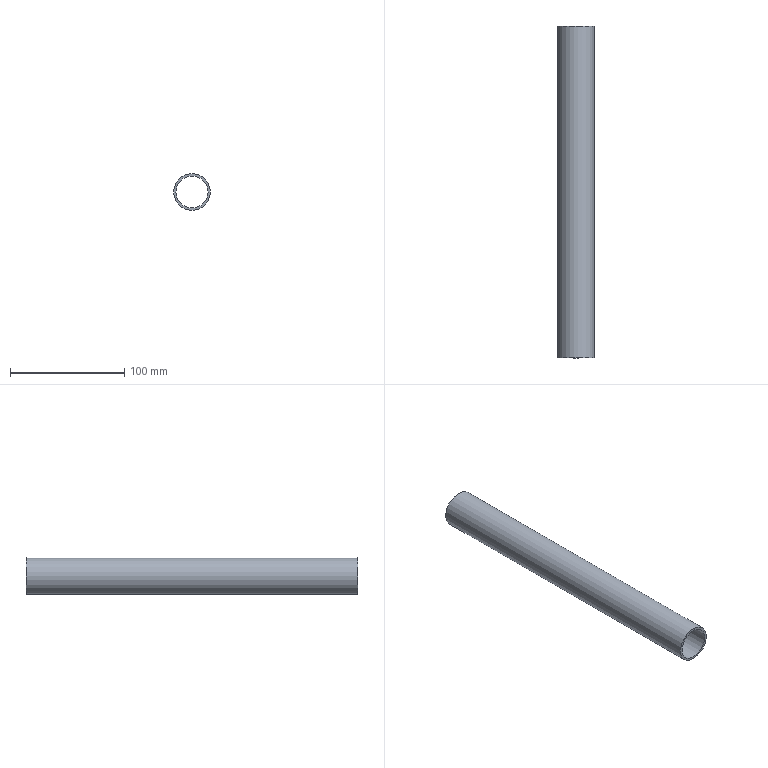Part | STEP file | 1-56.16 | 1 solid | 4 faces | box 32 x 290 x 32 mm | volume 54664 mm3 | plane 2 | cylinder 2 | commonest cylinder face diameters 28 x1 32 x1
STEP:
#1=CARTESIAN_POINT('',(0.,0.,0.));
#2=DIRECTION('',(0.,0.,1.));
#3=DIRECTION('',(1.,0.,0.));
#4=AXIS2_PLACEMENT_3D('',#1,#2,#3);
#5=CARTESIAN_POINT('',(16.,0.,0.));
#6=VERTEX_POINT('',#5);
#7=CARTESIAN_POINT('',(0.,0.,0.));
#8=DIRECTION('',(0.,-1.,0.));
#9=DIRECTION('',(1.,0.,0.));
#10=AXIS2_PLACEMENT_3D('',#7,#8,#9);
#11=CIRCLE('',#10,16.);
#12=CARTESIAN_POINT('',(-4.287,0.,0.));
#13=DIRECTION('',(0.,-1.,0.));
#14=DIRECTION('',(1.,0.,0.));
#15=AXIS2_PLACEMENT_3D('',#12,#13,#14);
#16=PLANE('',#15);
#17=CARTESIAN_POINT('',(4.287,0.));
#18=DIRECTION('',(1.,0.));
#19=AXIS2_PLACEMENT_2D('',#17,#18);
#20=CIRCLE('',#19,16.);
#21=(GEOMETRIC_REPRESENTATION_CONTEXT(2)PARAMETRIC_REPRESENTATION_CONTEXT()REPRESENTATION_CONTEXT('',''));
#22=DEFINITIONAL_REPRESENTATION('',(#20),#21);
#23=PCURVE('',#16,#22);
#24=CARTESIAN_POINT('',(0.,0.,0.));
#25=DIRECTION('',(0.,1.,0.));
#26=DIRECTION('',(1.,0.,0.));
#27=AXIS2_PLACEMENT_3D('',#24,#25,#26);
#28=CYLINDRICAL_SURFACE('',#27,16.);
#29=CARTESIAN_POINT('',(6.283,0.));
#30=DIRECTION('',(-1.,0.));
#31=VECTOR('',#30,1.);
#32=LINE('',#29,#31);
#33=(GEOMETRIC_REPRESENTATION_CONTEXT(2)PARAMETRIC_REPRESENTATION_CONTEXT()REPRESENTATION_CONTEXT('',''));
#34=DEFINITIONAL_REPRESENTATION('',(#32),#33);
#35=PCURVE('',#28,#34);
#36=SURFACE_CURVE('',#11,(#23,#35),.PCURVE_S1.);
#37=EDGE_CURVE('',#6,#6,#36,.T.);
#38=ORIENTED_EDGE('',*,*,#37,.T.);
#39=EDGE_LOOP('',(#38));
#40=FACE_BOUND('',#39,.T.);
#41=CARTESIAN_POINT('',(14.,0.,0.));
#42=VERTEX_POINT('',#41);
#43=CARTESIAN_POINT('',(0.,0.,0.));
#44=DIRECTION('',(0.,1.,0.));
#45=DIRECTION('',(1.,0.,0.));
#46=AXIS2_PLACEMENT_3D('',#43,#44,#45);
#47=CIRCLE('',#46,14.);
#48=CARTESIAN_POINT('',(18.287,0.));
#49=CARTESIAN_POINT('',(18.287,-24.249));
#50=CARTESIAN_POINT('',(-2.713,-12.124));
#51=CARTESIAN_POINT('',(-23.713,0.));
#52=CARTESIAN_POINT('',(-2.713,12.124));
#53=CARTESIAN_POINT('',(18.287,24.249));
#54=CARTESIAN_POINT('',(18.287,0.));
#55=(BOUNDED_CURVE()B_SPLINE_CURVE(2,(#48,#49,#50,#51,#52,#53,#54),.UNSPECIFIED.,.T.,.F.)B_SPLINE_CURVE_WITH_KNOTS((1,2,2,2,2,1),(-2.094,0.,2.094,4.189,6.283,8.378),.UNSPECIFIED.)CURVE()GEOMETRIC_REPRESENTATION_ITEM()RATIONAL_B_SPLINE_CURVE((1.,0.5,1.,0.5,1.,0.5,1.))REPRESENTATION_ITEM(''));
#56=(GEOMETRIC_REPRESENTATION_CONTEXT(2)PARAMETRIC_REPRESENTATION_CONTEXT()REPRESENTATION_CONTEXT('',''));
#57=DEFINITIONAL_REPRESENTATION('',(#55),#56);
#58=PCURVE('',#16,#57);
#59=CARTESIAN_POINT('',(0.,0.,0.));
#60=DIRECTION('',(0.,1.,0.));
#61=DIRECTION('',(1.,0.,0.));
#62=AXIS2_PLACEMENT_3D('',#59,#60,#61);
#63=CYLINDRICAL_SURFACE('',#62,14.);
#64=CARTESIAN_POINT('',(0.,0.));
#65=DIRECTION('',(1.,0.));
#66=VECTOR('',#65,1.);
#67=LINE('',#64,#66);
#68=(GEOMETRIC_REPRESENTATION_CONTEXT(2)PARAMETRIC_REPRESENTATION_CONTEXT()REPRESENTATION_CONTEXT('',''));
#69=DEFINITIONAL_REPRESENTATION('',(#67),#68);
#70=PCURVE('',#63,#69);
#71=SURFACE_CURVE('',#47,(#58,#70),.PCURVE_S1.);
#72=EDGE_CURVE('',#42,#42,#71,.T.);
#73=ORIENTED_EDGE('',*,*,#72,.T.);
#74=EDGE_LOOP('',(#73));
#75=FACE_BOUND('',#74,.T.);
#76=ADVANCED_FACE('',(#40,#75),#16,.T.);
#77=CARTESIAN_POINT('',(16.,290.,0.));
#78=VERTEX_POINT('',#77);
#79=CARTESIAN_POINT('',(0.,290.,0.));
#80=DIRECTION('',(0.,-1.,0.));
#81=DIRECTION('',(1.,0.,0.));
#82=AXIS2_PLACEMENT_3D('',#79,#80,#81);
#83=CIRCLE('',#82,16.);
#84=CARTESIAN_POINT('',(-4.287,290.,0.));
#85=DIRECTION('',(0.,-1.,0.));
#86=DIRECTION('',(1.,0.,0.));
#87=AXIS2_PLACEMENT_3D('',#84,#85,#86);
#88=PLANE('',#87);
#89=CARTESIAN_POINT('',(4.287,0.));
#90=DIRECTION('',(1.,0.));
#91=AXIS2_PLACEMENT_2D('',#89,#90);
#92=CIRCLE('',#91,16.);
#93=(GEOMETRIC_REPRESENTATION_CONTEXT(2)PARAMETRIC_REPRESENTATION_CONTEXT()REPRESENTATION_CONTEXT('',''));
#94=DEFINITIONAL_REPRESENTATION('',(#92),#93);
#95=PCURVE('',#88,#94);
#96=CARTESIAN_POINT('',(6.283,290.));
#97=DIRECTION('',(-1.,0.));
#98=VECTOR('',#97,1.);
#99=LINE('',#96,#98);
#100=(GEOMETRIC_REPRESENTATION_CONTEXT(2)PARAMETRIC_REPRESENTATION_CONTEXT()REPRESENTATION_CONTEXT('',''));
#101=DEFINITIONAL_REPRESENTATION('',(#99),#100);
#102=PCURVE('',#28,#101);
#103=SURFACE_CURVE('',#83,(#95,#102),.PCURVE_S1.);
#104=EDGE_CURVE('',#78,#78,#103,.T.);
#105=ORIENTED_EDGE('',*,*,#104,.T.);
#106=EDGE_LOOP('',(#105));
#107=FACE_BOUND('',#106,.F.);
#108=CARTESIAN_POINT('',(14.,290.,0.));
#109=VERTEX_POINT('',#108);
#110=CARTESIAN_POINT('',(0.,290.,0.));
#111=DIRECTION('',(0.,1.,0.));
#112=DIRECTION('',(1.,0.,0.));
#113=AXIS2_PLACEMENT_3D('',#110,#111,#112);
#114=CIRCLE('',#113,14.);
#115=CARTESIAN_POINT('',(18.287,0.));
#116=CARTESIAN_POINT('',(18.287,-24.249));
#117=CARTESIAN_POINT('',(-2.713,-12.124));
#118=CARTESIAN_POINT('',(-23.713,0.));
#119=CARTESIAN_POINT('',(-2.713,12.124));
#120=CARTESIAN_POINT('',(18.287,24.249));
#121=CARTESIAN_POINT('',(18.287,0.));
#122=(BOUNDED_CURVE()B_SPLINE_CURVE(2,(#115,#116,#117,#118,#119,#120,#121),.UNSPECIFIED.,.T.,.F.)B_SPLINE_CURVE_WITH_KNOTS((1,2,2,2,2,1),(-2.094,0.,2.094,4.189,6.283,8.378),.UNSPECIFIED.)CURVE()GEOMETRIC_REPRESENTATION_ITEM()RATIONAL_B_SPLINE_CURVE((1.,0.5,1.,0.5,1.,0.5,1.))REPRESENTATION_ITEM(''));
#123=(GEOMETRIC_REPRESENTATION_CONTEXT(2)PARAMETRIC_REPRESENTATION_CONTEXT()REPRESENTATION_CONTEXT('',''));
#124=DEFINITIONAL_REPRESENTATION('',(#122),#123);
#125=PCURVE('',#88,#124);
#126=CARTESIAN_POINT('',(0.,290.));
#127=DIRECTION('',(1.,0.));
#128=VECTOR('',#127,1.);
#129=LINE('',#126,#128);
#130=(GEOMETRIC_REPRESENTATION_CONTEXT(2)PARAMETRIC_REPRESENTATION_CONTEXT()REPRESENTATION_CONTEXT('',''));
#131=DEFINITIONAL_REPRESENTATION('',(#129),#130);
#132=PCURVE('',#63,#131);
#133=SURFACE_CURVE('',#114,(#125,#132),.PCURVE_S1.);
#134=EDGE_CURVE('',#109,#109,#133,.T.);
#135=ORIENTED_EDGE('',*,*,#134,.T.);
#136=EDGE_LOOP('',(#135));
#137=FACE_BOUND('',#136,.F.);
#138=ADVANCED_FACE('',(#107,#137),#88,.F.);
#139=CARTESIAN_POINT('',(16.,0.,0.));
#140=DIRECTION('',(0.,1.,0.));
#141=VECTOR('',#140,1.);
#142=LINE('',#139,#141);
#143=CARTESIAN_POINT('',(6.283,0.));
#144=DIRECTION('',(0.,1.));
#145=VECTOR('',#144,1.);
#146=LINE('',#143,#145);
#147=(GEOMETRIC_REPRESENTATION_CONTEXT(2)PARAMETRIC_REPRESENTATION_CONTEXT()REPRESENTATION_CONTEXT('',''));
#148=DEFINITIONAL_REPRESENTATION('',(#146),#147);
#149=PCURVE('',#28,#148);
#150=CARTESIAN_POINT('',(0.,0.));
#151=DIRECTION('',(0.,1.));
#152=VECTOR('',#151,1.);
#153=LINE('',#150,#152);
#154=(GEOMETRIC_REPRESENTATION_CONTEXT(2)PARAMETRIC_REPRESENTATION_CONTEXT()REPRESENTATION_CONTEXT('',''));
#155=DEFINITIONAL_REPRESENTATION('',(#153),#154);
#156=PCURVE('',#28,#155);
#157=SEAM_CURVE('',#142,(#149,#156),.PCURVE_S1.);
#158=EDGE_CURVE('',#6,#78,#157,.T.);
#159=ORIENTED_EDGE('',*,*,#158,.T.);
#160=ORIENTED_EDGE('',*,*,#104,.T.);
#161=ORIENTED_EDGE('',*,*,#158,.F.);
#162=ORIENTED_EDGE('',*,*,#37,.F.);
#163=EDGE_LOOP('',(#159,#160,#161,#162));
#164=FACE_BOUND('',#163,.T.);
#165=ADVANCED_FACE('',(#164),#28,.T.);
#166=ORIENTED_EDGE('',*,*,#72,.T.);
#167=CARTESIAN_POINT('',(14.,0.,0.));
#168=DIRECTION('',(0.,1.,0.));
#169=VECTOR('',#168,1.);
#170=LINE('',#167,#169);
#171=CARTESIAN_POINT('',(6.283,0.));
#172=DIRECTION('',(0.,1.));
#173=VECTOR('',#172,1.);
#174=LINE('',#171,#173);
#175=(GEOMETRIC_REPRESENTATION_CONTEXT(2)PARAMETRIC_REPRESENTATION_CONTEXT()REPRESENTATION_CONTEXT('',''));
#176=DEFINITIONAL_REPRESENTATION('',(#174),#175);
#177=PCURVE('',#63,#176);
#178=CARTESIAN_POINT('',(0.,0.));
#179=DIRECTION('',(0.,1.));
#180=VECTOR('',#179,1.);
#181=LINE('',#178,#180);
#182=(GEOMETRIC_REPRESENTATION_CONTEXT(2)PARAMETRIC_REPRESENTATION_CONTEXT()REPRESENTATION_CONTEXT('',''));
#183=DEFINITIONAL_REPRESENTATION('',(#181),#182);
#184=PCURVE('',#63,#183);
#185=SEAM_CURVE('',#170,(#177,#184),.PCURVE_S1.);
#186=EDGE_CURVE('',#42,#109,#185,.T.);
#187=ORIENTED_EDGE('',*,*,#186,.T.);
#188=ORIENTED_EDGE('',*,*,#134,.F.);
#189=ORIENTED_EDGE('',*,*,#186,.F.);
#190=EDGE_LOOP('',(#166,#187,#188,#189));
#191=FACE_BOUND('',#190,.F.);
#192=ADVANCED_FACE('',(#191),#63,.F.);
#193=CLOSED_SHELL('',(#76,#138,#165,#192));
#194=MANIFOLD_SOLID_BREP('',#193);
#195=(LENGTH_UNIT()NAMED_UNIT(*)SI_UNIT(.MILLI.,.METRE.));
#196=UNCERTAINTY_MEASURE_WITH_UNIT(LENGTH_MEASURE(0.0000001),#195,'','');
#197=(NAMED_UNIT(*)PLANE_ANGLE_UNIT()SI_UNIT($,.RADIAN.));
#198=(NAMED_UNIT(*)SI_UNIT($,.STERADIAN.)SOLID_ANGLE_UNIT());
#199=(GEOMETRIC_REPRESENTATION_CONTEXT(3)GLOBAL_UNCERTAINTY_ASSIGNED_CONTEXT((#196))GLOBAL_UNIT_ASSIGNED_CONTEXT((#195,#197,#198))REPRESENTATION_CONTEXT('',''));
#200=ADVANCED_BREP_SHAPE_REPRESENTATION('',(#4,#194),#199);